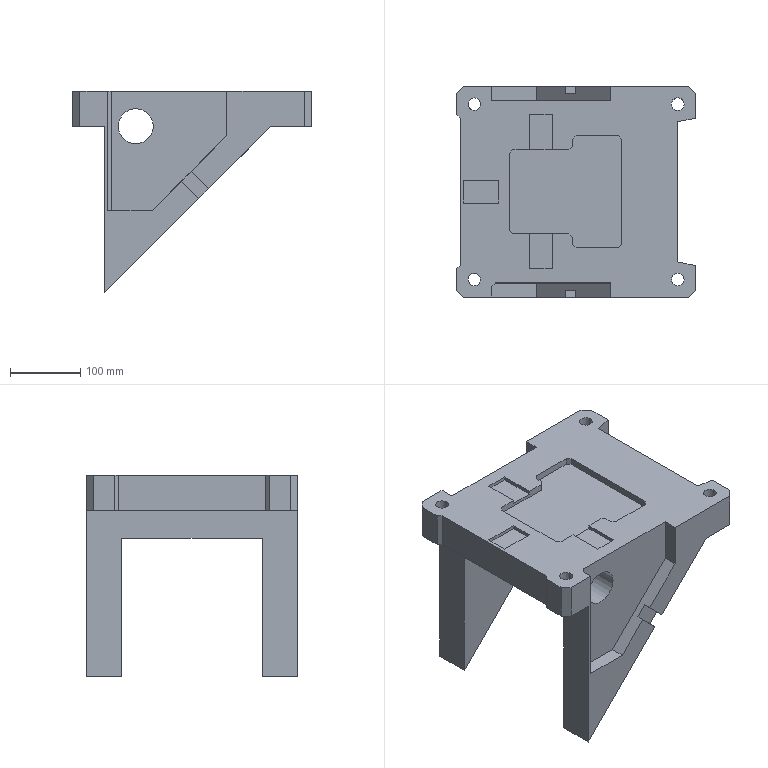Part | NX | features solid 2 | 1 solid | 88 faces | box 340 x 300 x 287.267 mm | volume 6379745 mm3 | plane 79 | cylinder 9 | commonest cylinder face diameters 18 x4 22 x4 50 x1